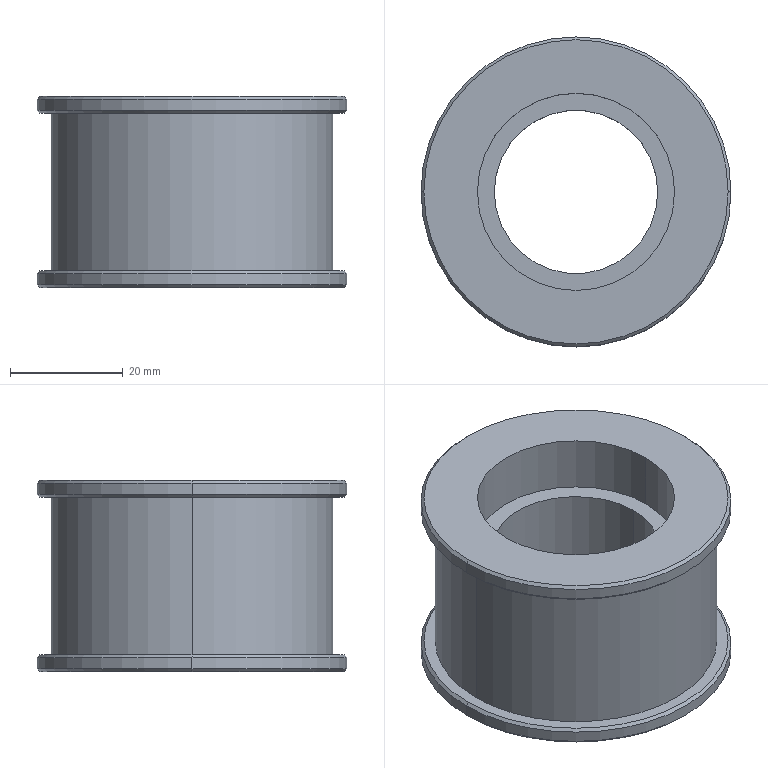Part | STEP file | CON-004 | 1 solid | 26 faces | box 55 x 55 x 34 mm | volume 40657 mm3 | cylinder 12 | cone 8 | plane 6 | commonest cylinder face diameters 35 x4 55 x4 29 x2 50 x2